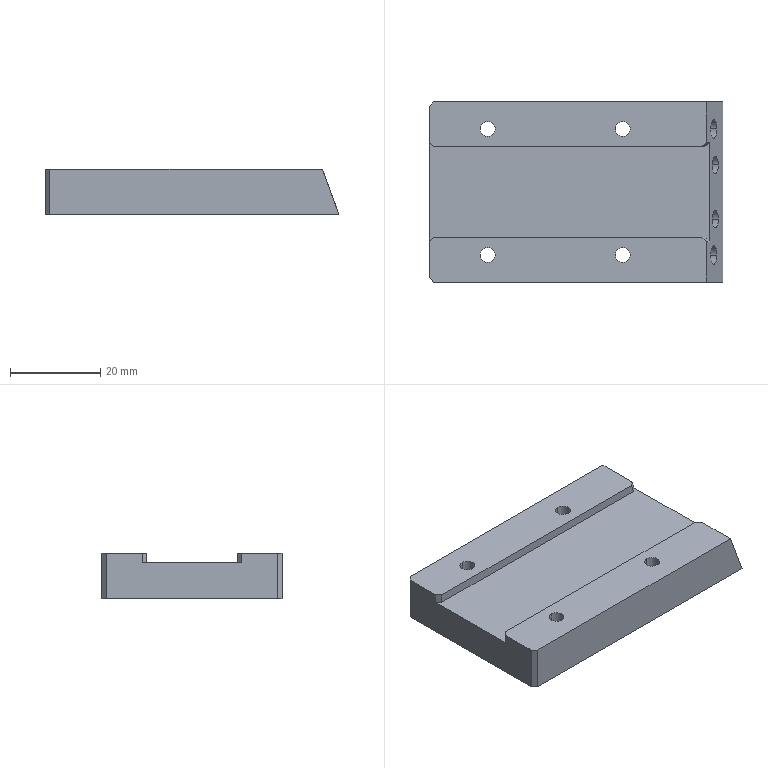NC program | NX | posted with a generic post | part box 65.2 x 40 x 10 mm
Whole program:
N10 G17 G21 G94 G90
(ZLEVEL_PROFILE_1_COPY , TOOL : D6JING)
N12 T16 M6
N14 G54
N16 G17 G0 G90 X-32.258 Y23.539 S6500 M3
N18 G43 Z30. H16
N20 Z-9.
N22 G94 G1 Z-10. F1000.
N24 X-32.12 Y23.3
N26 G3 X-31.6 Y23. R0.6
N28 G1 X32.599
N30 G2 X35.598 Y20. R3.
N32 G1 Y-19.998
N34 G2 X32.596 Y-23. R3.002
N36 G1 X-31.6
N38 G2 X-33.721 Y-22.121 R3.
N40 G1 X-34.721 Y-21.121
N42 G2 X-35.6 Y-19. R3.
N44 G1 Y19.
N46 G2 X-34.721 Y21.121 R3.
N48 G1 X-33.721 Y22.121
N50 G2 X-31.6 Y23. R3.
N52 G3 X-31.08 Y23.3 R0.6
N54 G1 X-30.907 Y23.6
N56 Z-9.
N58 G0 Z30.
(FLOOR_WALL , TOOL : D6JING)
N60 X-36.6 Y7.731
N62 Z-1.
N64 G1 Z-2. F1250.
N66 X-36.12 Y6.899
N68 G3 X-35.6 Y6.599 R0.6
N70 G1 X32.688
N72 Y3.959
N74 X-35.6
N76 Y1.319
N78 X32.688
N80 Y-1.32
N82 X-35.6
N84 Y-3.96
N86 X32.688
N88 Y-6.6
N90 X-35.6
N92 G2 X-36.12 Y-6.3 R0.6
N94 G1 X-36.6 Y-5.468
N96 Z-1.
N98 G0 Z30.
N100 X-36.7 Y-9.619
N102 Z-1.
N104 G1 Z-2.
N106 X-36.17 Y-9.761
N108 G3 X-35.59 Y-9.606 R0.6
N110 G1 X-32.884 Y-6.9
N112 X29.852
N114 X32.688 Y-9.565
N116 G3 X33.272 Y-9.702 R0.6
N118 G1 X33.788 Y-9.547
N120 Z-1.
N122 G0 Z30.
N124 Y9.547
N126 Z-1.
N128 G1 Z-2.
N130 X33.272 Y9.702
N132 G3 X32.688 Y9.565 R0.6
N134 G1 X29.852 Y6.9
N136 X-32.884
N138 X-35.59 Y9.606
N140 G3 X-36.17 Y9.761 R0.6
N142 G1 X-36.7 Y9.619
N144 Z-1.
N146 G0 Z30.
N148 M5
(刀补16 , TOOL : D6JING)
N150 M6
N152 G54
N154 G17 G0 G90 X-36.741 Y-9.661 S9500 M3
N156 G43 Z30. H16
N158 Z-1.
N160 G94 G1 Z-2. F1250.
N162 G41 X-36.65 Y-9.703 D16
N164 X-36.17 Y-9.832
N166 G3 X-35.59 Y-9.677 R0.6
N168 G1 X-32.863 Y-6.95
N170 X29.832
N172 X32.688 Y-9.634
N174 G3 X33.272 Y-9.771 R0.6
N176 G1 X33.738 Y-9.63
N178 G40
N180 X33.828 Y-9.585
N182 Z-1.
N184 G0 Z30.
N186 Y9.585
N188 Z-1.
N190 G1 Z-2.
N192 G41 X33.738 Y9.63
N194 X33.272 Y9.771
N196 G3 X32.688 Y9.634 R0.6
N198 G1 X29.832 Y6.95
N200 X-32.863
N202 X-35.6 Y9.687
N204 G3 X-36.18 Y9.842 R0.6
N206 G1 X-36.65 Y9.716
N208 G40
N210 X-36.741 Y9.674
N212 Z-1.
N214 G0 Z30.
N216 M5
N218 M2